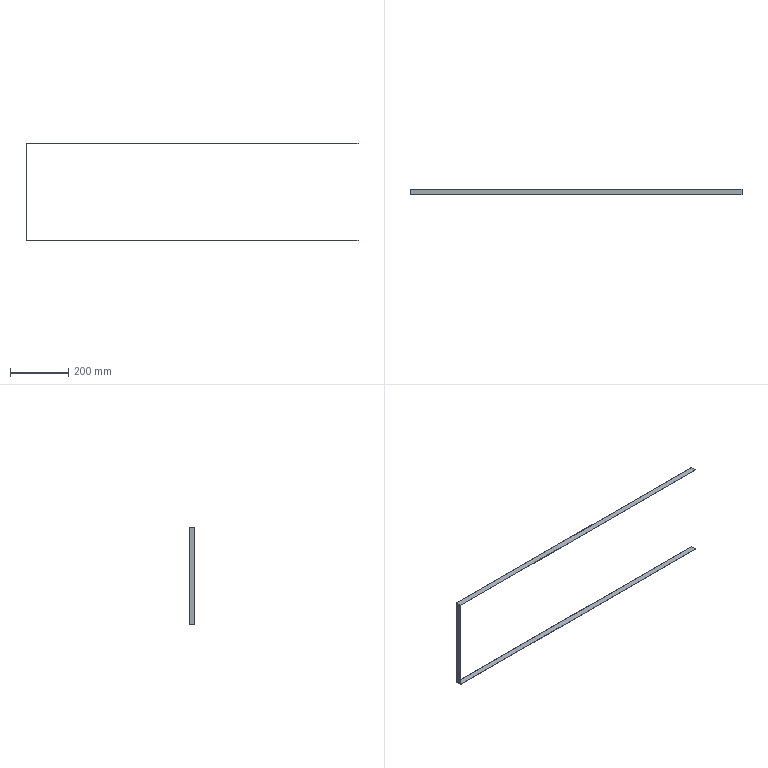Part | STEP file | 1013-3.stp.STEP | 1 solid | 10 faces | box 1140 x 20 x 333.2 mm | volume 31334 mm3 | plane 10
STEP:
#1=CARTESIAN_POINT('',(569.5,31.5,166.));
#2=VERTEX_POINT('',#1);
#3=CARTESIAN_POINT('',(-569.5,31.5,166.));
#4=VERTEX_POINT('',#3);
#5=CARTESIAN_POINT('',(569.5,31.5,166.));
#6=DIRECTION('',(-1.,0.,0.));
#7=VECTOR('',#6,1000.);
#8=LINE('',#5,#7);
#9=EDGE_CURVE('',#2,#4,#8,.T.);
#10=ORIENTED_EDGE('',*,*,#9,.F.);
#11=CARTESIAN_POINT('',(569.5,11.5,166.));
#12=VERTEX_POINT('',#11);
#13=CARTESIAN_POINT('',(569.5,11.5,166.));
#14=DIRECTION('',(0.,1.,0.));
#15=VECTOR('',#14,1000.);
#16=LINE('',#13,#15);
#17=EDGE_CURVE('',#12,#2,#16,.T.);
#18=ORIENTED_EDGE('',*,*,#17,.F.);
#19=CARTESIAN_POINT('',(-569.5,11.5,166.));
#20=VERTEX_POINT('',#19);
#21=CARTESIAN_POINT('',(-569.5,11.5,166.));
#22=DIRECTION('',(1.,0.,0.));
#23=VECTOR('',#22,1000.);
#24=LINE('',#21,#23);
#25=EDGE_CURVE('',#20,#12,#24,.T.);
#26=ORIENTED_EDGE('',*,*,#25,.F.);
#27=CARTESIAN_POINT('',(-569.5,31.5,166.));
#28=DIRECTION('',(0.,-1.,0.));
#29=VECTOR('',#28,1000.);
#30=LINE('',#27,#29);
#31=EDGE_CURVE('',#4,#20,#30,.T.);
#32=ORIENTED_EDGE('',*,*,#31,.F.);
#33=EDGE_LOOP('',(#10,#18,#26,#32));
#34=FACE_OUTER_BOUND('',#33,.T.);
#35=CARTESIAN_POINT('',(-569.5,-4.5,166.));
#36=DIRECTION('',(0.,0.,1.));
#37=DIRECTION('',(1.,0.,0.));
#38=AXIS2_PLACEMENT_3D('',#35,#36,#37);
#39=PLANE('',#38);
#40=ADVANCED_FACE('',(#34),#39,.F.);
#41=CARTESIAN_POINT('',(-569.5,11.5,-166.));
#42=VERTEX_POINT('',#41);
#43=CARTESIAN_POINT('',(-569.5,11.5,-166.));
#44=DIRECTION('',(0.,0.,1.));
#45=VECTOR('',#44,1000.);
#46=LINE('',#43,#45);
#47=EDGE_CURVE('',#42,#20,#46,.T.);
#48=ORIENTED_EDGE('',*,*,#47,.F.);
#49=CARTESIAN_POINT('',(-569.5,31.5,-166.));
#50=VERTEX_POINT('',#49);
#51=CARTESIAN_POINT('',(-569.5,31.5,-166.));
#52=DIRECTION('',(0.,-1.,0.));
#53=VECTOR('',#52,1000.);
#54=LINE('',#51,#53);
#55=EDGE_CURVE('',#50,#42,#54,.T.);
#56=ORIENTED_EDGE('',*,*,#55,.F.);
#57=CARTESIAN_POINT('',(-569.5,31.5,166.));
#58=DIRECTION('',(0.,0.,-1.));
#59=VECTOR('',#58,1000.);
#60=LINE('',#57,#59);
#61=EDGE_CURVE('',#4,#50,#60,.T.);
#62=ORIENTED_EDGE('',*,*,#61,.F.);
#63=ORIENTED_EDGE('',*,*,#31,.T.);
#64=EDGE_LOOP('',(#48,#56,#62,#63));
#65=FACE_OUTER_BOUND('',#64,.T.);
#66=CARTESIAN_POINT('',(-569.5,-4.5,166.));
#67=DIRECTION('',(-1.,0.,0.));
#68=DIRECTION('',(0.,0.,1.));
#69=AXIS2_PLACEMENT_3D('',#66,#67,#68);
#70=PLANE('',#69);
#71=ADVANCED_FACE('',(#65),#70,.F.);
#72=CARTESIAN_POINT('',(-570.1,31.5,166.6));
#73=VERTEX_POINT('',#72);
#74=CARTESIAN_POINT('',(-570.1,31.5,-166.6));
#75=VERTEX_POINT('',#74);
#76=CARTESIAN_POINT('',(-570.1,31.5,166.6));
#77=DIRECTION('',(0.,0.,-1.));
#78=VECTOR('',#77,1000.);
#79=LINE('',#76,#78);
#80=EDGE_CURVE('',#73,#75,#79,.T.);
#81=ORIENTED_EDGE('',*,*,#80,.F.);
#82=CARTESIAN_POINT('',(569.5,31.5,166.6));
#83=VERTEX_POINT('',#82);
#84=CARTESIAN_POINT('',(569.5,31.5,166.6));
#85=DIRECTION('',(-1.,0.,0.));
#86=VECTOR('',#85,1000.);
#87=LINE('',#84,#86);
#88=EDGE_CURVE('',#83,#73,#87,.T.);
#89=ORIENTED_EDGE('',*,*,#88,.F.);
#90=CARTESIAN_POINT('',(569.5,31.5,166.));
#91=DIRECTION('',(0.,0.,1.));
#92=VECTOR('',#91,1000.);
#93=LINE('',#90,#92);
#94=EDGE_CURVE('',#2,#83,#93,.T.);
#95=ORIENTED_EDGE('',*,*,#94,.F.);
#96=ORIENTED_EDGE('',*,*,#9,.T.);
#97=ORIENTED_EDGE('',*,*,#61,.T.);
#98=CARTESIAN_POINT('',(569.5,31.5,-166.));
#99=VERTEX_POINT('',#98);
#100=CARTESIAN_POINT('',(569.5,31.5,-166.));
#101=DIRECTION('',(-1.,0.,0.));
#102=VECTOR('',#101,1000.);
#103=LINE('',#100,#102);
#104=EDGE_CURVE('',#99,#50,#103,.T.);
#105=ORIENTED_EDGE('',*,*,#104,.F.);
#106=CARTESIAN_POINT('',(569.5,31.5,-166.6));
#107=VERTEX_POINT('',#106);
#108=CARTESIAN_POINT('',(569.5,31.5,-166.));
#109=DIRECTION('',(0.,0.,-1.));
#110=VECTOR('',#109,1000.);
#111=LINE('',#108,#110);
#112=EDGE_CURVE('',#99,#107,#111,.T.);
#113=ORIENTED_EDGE('',*,*,#112,.T.);
#114=CARTESIAN_POINT('',(-570.1,31.5,-166.6));
#115=DIRECTION('',(1.,0.,0.));
#116=VECTOR('',#115,1000.);
#117=LINE('',#114,#116);
#118=EDGE_CURVE('',#75,#107,#117,.T.);
#119=ORIENTED_EDGE('',*,*,#118,.F.);
#120=EDGE_LOOP('',(#81,#89,#95,#96,#97,#105,#113,#119));
#121=FACE_OUTER_BOUND('',#120,.T.);
#122=CARTESIAN_POINT('',(569.5,31.5,166.));
#123=DIRECTION('',(0.,1.,0.));
#124=DIRECTION('',(1.,0.,0.));
#125=AXIS2_PLACEMENT_3D('',#122,#123,#124);
#126=PLANE('',#125);
#127=ADVANCED_FACE('',(#121),#126,.T.);
#128=CARTESIAN_POINT('',(569.5,11.5,-166.6));
#129=VERTEX_POINT('',#128);
#130=CARTESIAN_POINT('',(569.5,11.5,-166.6));
#131=DIRECTION('',(0.,1.,0.));
#132=VECTOR('',#131,1000.);
#133=LINE('',#130,#132);
#134=EDGE_CURVE('',#129,#107,#133,.T.);
#135=ORIENTED_EDGE('',*,*,#134,.F.);
#136=CARTESIAN_POINT('',(-570.1,11.5,-166.6));
#137=VERTEX_POINT('',#136);
#138=CARTESIAN_POINT('',(-570.1,11.5,-166.6));
#139=DIRECTION('',(1.,0.,0.));
#140=VECTOR('',#139,1000.);
#141=LINE('',#138,#140);
#142=EDGE_CURVE('',#137,#129,#141,.T.);
#143=ORIENTED_EDGE('',*,*,#142,.F.);
#144=CARTESIAN_POINT('',(-570.1,31.5,-166.6));
#145=DIRECTION('',(0.,-1.,0.));
#146=VECTOR('',#145,1000.);
#147=LINE('',#144,#146);
#148=EDGE_CURVE('',#75,#137,#147,.T.);
#149=ORIENTED_EDGE('',*,*,#148,.F.);
#150=ORIENTED_EDGE('',*,*,#118,.T.);
#151=EDGE_LOOP('',(#135,#143,#149,#150));
#152=FACE_OUTER_BOUND('',#151,.T.);
#153=CARTESIAN_POINT('',(-569.5,-4.5,-166.6));
#154=DIRECTION('',(0.,0.,1.));
#155=DIRECTION('',(1.,0.,0.));
#156=AXIS2_PLACEMENT_3D('',#153,#154,#155);
#157=PLANE('',#156);
#158=ADVANCED_FACE('',(#152),#157,.F.);
#159=ORIENTED_EDGE('',*,*,#148,.T.);
#160=CARTESIAN_POINT('',(-570.1,11.5,166.6));
#161=VERTEX_POINT('',#160);
#162=CARTESIAN_POINT('',(-570.1,11.5,-166.6));
#163=DIRECTION('',(0.,0.,1.));
#164=VECTOR('',#163,1000.);
#165=LINE('',#162,#164);
#166=EDGE_CURVE('',#137,#161,#165,.T.);
#167=ORIENTED_EDGE('',*,*,#166,.T.);
#168=CARTESIAN_POINT('',(-570.1,11.5,166.6));
#169=DIRECTION('',(0.,1.,0.));
#170=VECTOR('',#169,1000.);
#171=LINE('',#168,#170);
#172=EDGE_CURVE('',#161,#73,#171,.T.);
#173=ORIENTED_EDGE('',*,*,#172,.T.);
#174=ORIENTED_EDGE('',*,*,#80,.T.);
#175=EDGE_LOOP('',(#159,#167,#173,#174));
#176=FACE_OUTER_BOUND('',#175,.T.);
#177=CARTESIAN_POINT('',(-570.1,-4.5,166.));
#178=DIRECTION('',(-1.,0.,0.));
#179=DIRECTION('',(0.,0.,1.));
#180=AXIS2_PLACEMENT_3D('',#177,#178,#179);
#181=PLANE('',#180);
#182=ADVANCED_FACE('',(#176),#181,.T.);
#183=CARTESIAN_POINT('',(569.5,11.5,166.6));
#184=VERTEX_POINT('',#183);
#185=CARTESIAN_POINT('',(569.5,11.5,166.6));
#186=DIRECTION('',(0.,1.,0.));
#187=VECTOR('',#186,1000.);
#188=LINE('',#185,#187);
#189=EDGE_CURVE('',#184,#83,#188,.T.);
#190=ORIENTED_EDGE('',*,*,#189,.T.);
#191=ORIENTED_EDGE('',*,*,#88,.T.);
#192=ORIENTED_EDGE('',*,*,#172,.F.);
#193=CARTESIAN_POINT('',(-570.1,11.5,166.6));
#194=DIRECTION('',(1.,0.,0.));
#195=VECTOR('',#194,1000.);
#196=LINE('',#193,#195);
#197=EDGE_CURVE('',#161,#184,#196,.T.);
#198=ORIENTED_EDGE('',*,*,#197,.T.);
#199=EDGE_LOOP('',(#190,#191,#192,#198));
#200=FACE_OUTER_BOUND('',#199,.T.);
#201=CARTESIAN_POINT('',(-569.5,-4.5,166.6));
#202=DIRECTION('',(0.,0.,1.));
#203=DIRECTION('',(1.,0.,0.));
#204=AXIS2_PLACEMENT_3D('',#201,#202,#203);
#205=PLANE('',#204);
#206=ADVANCED_FACE('',(#200),#205,.T.);
#207=ORIENTED_EDGE('',*,*,#25,.T.);
#208=CARTESIAN_POINT('',(569.5,11.5,166.));
#209=DIRECTION('',(0.,0.,1.));
#210=VECTOR('',#209,1000.);
#211=LINE('',#208,#210);
#212=EDGE_CURVE('',#12,#184,#211,.T.);
#213=ORIENTED_EDGE('',*,*,#212,.T.);
#214=ORIENTED_EDGE('',*,*,#197,.F.);
#215=ORIENTED_EDGE('',*,*,#166,.F.);
#216=ORIENTED_EDGE('',*,*,#142,.T.);
#217=CARTESIAN_POINT('',(569.5,11.5,-166.));
#218=VERTEX_POINT('',#217);
#219=CARTESIAN_POINT('',(569.5,11.5,-166.));
#220=DIRECTION('',(0.,0.,-1.));
#221=VECTOR('',#220,1000.);
#222=LINE('',#219,#221);
#223=EDGE_CURVE('',#218,#129,#222,.T.);
#224=ORIENTED_EDGE('',*,*,#223,.F.);
#225=CARTESIAN_POINT('',(-569.5,11.5,-166.));
#226=DIRECTION('',(1.,0.,0.));
#227=VECTOR('',#226,1000.);
#228=LINE('',#225,#227);
#229=EDGE_CURVE('',#42,#218,#228,.T.);
#230=ORIENTED_EDGE('',*,*,#229,.F.);
#231=ORIENTED_EDGE('',*,*,#47,.T.);
#232=EDGE_LOOP('',(#207,#213,#214,#215,#216,#224,#230,#231));
#233=FACE_OUTER_BOUND('',#232,.T.);
#234=CARTESIAN_POINT('',(-569.5,11.5,166.));
#235=DIRECTION('',(0.,-1.,0.));
#236=DIRECTION('',(0.,0.,-1.));
#237=AXIS2_PLACEMENT_3D('',#234,#235,#236);
#238=PLANE('',#237);
#239=ADVANCED_FACE('',(#233),#238,.T.);
#240=ORIENTED_EDGE('',*,*,#229,.T.);
#241=CARTESIAN_POINT('',(569.5,11.5,-166.));
#242=DIRECTION('',(0.,1.,0.));
#243=VECTOR('',#242,1000.);
#244=LINE('',#241,#243);
#245=EDGE_CURVE('',#218,#99,#244,.T.);
#246=ORIENTED_EDGE('',*,*,#245,.T.);
#247=ORIENTED_EDGE('',*,*,#104,.T.);
#248=ORIENTED_EDGE('',*,*,#55,.T.);
#249=EDGE_LOOP('',(#240,#246,#247,#248));
#250=FACE_OUTER_BOUND('',#249,.T.);
#251=CARTESIAN_POINT('',(-569.5,-4.5,-166.));
#252=DIRECTION('',(0.,0.,1.));
#253=DIRECTION('',(1.,0.,0.));
#254=AXIS2_PLACEMENT_3D('',#251,#252,#253);
#255=PLANE('',#254);
#256=ADVANCED_FACE('',(#250),#255,.T.);
#257=ORIENTED_EDGE('',*,*,#223,.T.);
#258=ORIENTED_EDGE('',*,*,#134,.T.);
#259=ORIENTED_EDGE('',*,*,#112,.F.);
#260=ORIENTED_EDGE('',*,*,#245,.F.);
#261=EDGE_LOOP('',(#257,#258,#259,#260));
#262=FACE_OUTER_BOUND('',#261,.T.);
#263=CARTESIAN_POINT('',(569.5,11.5,-166.));
#264=DIRECTION('',(-1.,0.,0.));
#265=DIRECTION('',(0.,0.,1.));
#266=AXIS2_PLACEMENT_3D('',#263,#264,#265);
#267=PLANE('',#266);
#268=ADVANCED_FACE('',(#262),#267,.F.);
#269=ORIENTED_EDGE('',*,*,#94,.T.);
#270=ORIENTED_EDGE('',*,*,#189,.F.);
#271=ORIENTED_EDGE('',*,*,#212,.F.);
#272=ORIENTED_EDGE('',*,*,#17,.T.);
#273=EDGE_LOOP('',(#269,#270,#271,#272));
#274=FACE_OUTER_BOUND('',#273,.T.);
#275=CARTESIAN_POINT('',(569.5,11.5,166.));
#276=DIRECTION('',(1.,0.,0.));
#277=DIRECTION('',(0.,1.,0.));
#278=AXIS2_PLACEMENT_3D('',#275,#276,#277);
#279=PLANE('',#278);
#280=ADVANCED_FACE('',(#274),#279,.T.);
#281=CLOSED_SHELL('',(#40,#71,#127,#158,#182,#206,#239,#256,#268,#280));
#282=MANIFOLD_SOLID_BREP('',#281);
#283=CARTESIAN_POINT('',(0.,0.,0.));
#284=DIRECTION('',(0.,0.,1.));
#285=DIRECTION('',(1.,0.,0.));
#286=AXIS2_PLACEMENT_3D('',#283,#284,#285);
#287=(LENGTH_UNIT()NAMED_UNIT(*)SI_UNIT(.MILLI.,.METRE.));
#288=UNCERTAINTY_MEASURE_WITH_UNIT(LENGTH_MEASURE(0.00001),#287,'','');
#289=(NAMED_UNIT(*)PLANE_ANGLE_UNIT()SI_UNIT($,.RADIAN.));
#290=(NAMED_UNIT(*)SI_UNIT($,.STERADIAN.)SOLID_ANGLE_UNIT());
#291=(GEOMETRIC_REPRESENTATION_CONTEXT(3)GLOBAL_UNCERTAINTY_ASSIGNED_CONTEXT((#288))GLOBAL_UNIT_ASSIGNED_CONTEXT((#287,#289,#290))REPRESENTATION_CONTEXT('',''));
#292=ADVANCED_BREP_SHAPE_REPRESENTATION('',(#282,#286),#291);